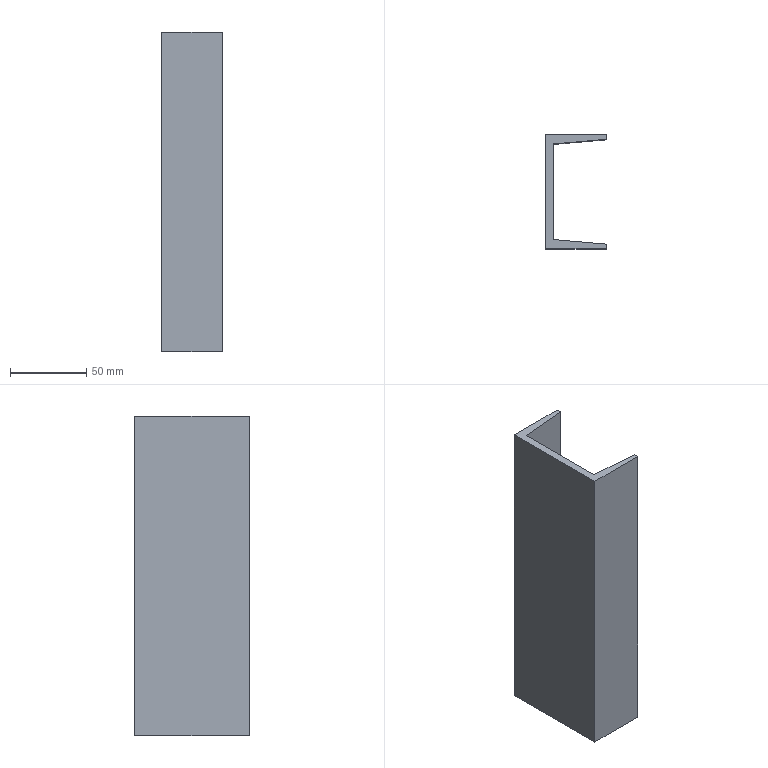Part | STEP file | BCC3 H13_7 | 1 solid | 12 faces | box 40 x 75 x 210 mm | volume 144819 mm3 | plane 10 | cylinder 2 | commonest cylinder face diameters 12 x2
STEP:
#1=CARTESIAN_POINT('',(0.,0.,0.));
#2=DIRECTION('',(0.,0.,1.));
#3=DIRECTION('',(1.,0.,0.));
#4=AXIS2_PLACEMENT_3D('',#1,#2,#3);
#5=CARTESIAN_POINT('',(20.,32.75,6.));
#6=VERTEX_POINT('',#5);
#7=CARTESIAN_POINT('',(20.,37.5,6.));
#8=VERTEX_POINT('',#7);
#9=CARTESIAN_POINT('',(20.,27.5,6.));
#10=DIRECTION('',(0.,1.,0.));
#11=VECTOR('',#10,1.);
#12=LINE('',#9,#11);
#13=CARTESIAN_POINT('',(20.,27.5,0.));
#14=DIRECTION('',(0.,1.,0.));
#15=DIRECTION('',(0.,0.,1.));
#16=AXIS2_PLACEMENT_3D('',#13,#14,#15);
#17=CYLINDRICAL_SURFACE('',#16,6.);
#18=CARTESIAN_POINT('',(6.283,0.));
#19=DIRECTION('',(0.,1.));
#20=VECTOR('',#19,1.);
#21=LINE('',#18,#20);
#22=(GEOMETRIC_REPRESENTATION_CONTEXT(2)PARAMETRIC_REPRESENTATION_CONTEXT()REPRESENTATION_CONTEXT('',''));
#23=DEFINITIONAL_REPRESENTATION('',(#21),#22);
#24=PCURVE('',#17,#23);
#25=CARTESIAN_POINT('',(20.,27.5,0.));
#26=DIRECTION('',(0.,1.,0.));
#27=DIRECTION('',(0.,0.,1.));
#28=AXIS2_PLACEMENT_3D('',#25,#26,#27);
#29=CYLINDRICAL_SURFACE('',#28,6.);
#30=CARTESIAN_POINT('',(0.,0.));
#31=DIRECTION('',(0.,1.));
#32=VECTOR('',#31,1.);
#33=LINE('',#30,#32);
#34=(GEOMETRIC_REPRESENTATION_CONTEXT(2)PARAMETRIC_REPRESENTATION_CONTEXT()REPRESENTATION_CONTEXT('',''));
#35=DEFINITIONAL_REPRESENTATION('',(#33),#34);
#36=PCURVE('',#29,#35);
#37=SURFACE_CURVE('',#12,(#24,#36),.PCURVE_S1.);
#38=EDGE_CURVE('',#6,#8,#37,.T.);
#39=ORIENTED_EDGE('',*,*,#38,.T.);
#40=CARTESIAN_POINT('',(20.,37.5,-6.));
#41=VERTEX_POINT('',#40);
#42=CARTESIAN_POINT('',(20.,37.5,0.));
#43=DIRECTION('',(0.,-1.,0.));
#44=DIRECTION('',(0.,0.,-1.));
#45=AXIS2_PLACEMENT_3D('',#42,#43,#44);
#46=CIRCLE('',#45,6.);
#47=CARTESIAN_POINT('',(9.425,10.));
#48=DIRECTION('',(-1.,0.));
#49=VECTOR('',#48,1.);
#50=LINE('',#47,#49);
#51=(GEOMETRIC_REPRESENTATION_CONTEXT(2)PARAMETRIC_REPRESENTATION_CONTEXT()REPRESENTATION_CONTEXT('',''));
#52=DEFINITIONAL_REPRESENTATION('',(#50),#51);
#53=PCURVE('',#17,#52);
#54=CARTESIAN_POINT('',(40.,37.5,105.));
#55=DIRECTION('',(0.,-1.,0.));
#56=DIRECTION('',(0.,0.,-1.));
#57=AXIS2_PLACEMENT_3D('',#54,#55,#56);
#58=PLANE('',#57);
#59=CARTESIAN_POINT('',(105.,-20.));
#60=DIRECTION('',(1.,0.));
#61=AXIS2_PLACEMENT_2D('',#59,#60);
#62=CIRCLE('',#61,6.);
#63=(GEOMETRIC_REPRESENTATION_CONTEXT(2)PARAMETRIC_REPRESENTATION_CONTEXT()REPRESENTATION_CONTEXT('',''));
#64=DEFINITIONAL_REPRESENTATION('',(#62),#63);
#65=PCURVE('',#58,#64);
#66=SURFACE_CURVE('',#46,(#53,#65),.PCURVE_S1.);
#67=EDGE_CURVE('',#8,#41,#66,.T.);
#68=ORIENTED_EDGE('',*,*,#67,.T.);
#69=CARTESIAN_POINT('',(20.,32.75,-6.));
#70=VERTEX_POINT('',#69);
#71=CARTESIAN_POINT('',(20.,27.5,-6.));
#72=DIRECTION('',(0.,1.,0.));
#73=VECTOR('',#72,1.);
#74=LINE('',#71,#73);
#75=CARTESIAN_POINT('',(3.142,0.));
#76=DIRECTION('',(0.,1.));
#77=VECTOR('',#76,1.);
#78=LINE('',#75,#77);
#79=(GEOMETRIC_REPRESENTATION_CONTEXT(2)PARAMETRIC_REPRESENTATION_CONTEXT()REPRESENTATION_CONTEXT('',''));
#80=DEFINITIONAL_REPRESENTATION('',(#78),#79);
#81=PCURVE('',#17,#80);
#82=CARTESIAN_POINT('',(3.142,0.));
#83=DIRECTION('',(0.,1.));
#84=VECTOR('',#83,1.);
#85=LINE('',#82,#84);
#86=(GEOMETRIC_REPRESENTATION_CONTEXT(2)PARAMETRIC_REPRESENTATION_CONTEXT()REPRESENTATION_CONTEXT('',''));
#87=DEFINITIONAL_REPRESENTATION('',(#85),#86);
#88=PCURVE('',#29,#87);
#89=SURFACE_CURVE('',#74,(#81,#88),.PCURVE_S1.);
#90=EDGE_CURVE('',#70,#41,#89,.T.);
#91=ORIENTED_EDGE('',*,*,#90,.F.);
#92=CARTESIAN_POINT('',(20.,32.75,6.));
#93=CARTESIAN_POINT('',(8.,31.7,6.));
#94=CARTESIAN_POINT('',(8.,31.7,-6.));
#95=CARTESIAN_POINT('',(20.,32.75,-6.));
#96=(BOUNDED_CURVE()B_SPLINE_CURVE(3,(#92,#93,#94,#95),.UNSPECIFIED.,.F.,.F.)B_SPLINE_CURVE_WITH_KNOTS((4,4),(1.571,4.712),.PIECEWISE_BEZIER_KNOTS.)CURVE()GEOMETRIC_REPRESENTATION_ITEM()RATIONAL_B_SPLINE_CURVE((1.,0.3333,0.3333,1.))REPRESENTATION_ITEM(''));
#97=CARTESIAN_POINT('',(6.283,5.25));
#98=CARTESIAN_POINT('',(6.253,5.234));
#99=CARTESIAN_POINT('',(6.19,5.201));
#100=CARTESIAN_POINT('',(6.085,5.147));
#101=CARTESIAN_POINT('',(5.972,5.089));
#102=CARTESIAN_POINT('',(5.848,5.028));
#103=CARTESIAN_POINT('',(5.713,4.966));
#104=CARTESIAN_POINT('',(5.567,4.904));
#105=CARTESIAN_POINT('',(5.412,4.847));
#106=CARTESIAN_POINT('',(5.246,4.796));
#107=CARTESIAN_POINT('',(5.073,4.757));
#108=CARTESIAN_POINT('',(4.894,4.731));
#109=CARTESIAN_POINT('',(4.712,4.722));
#110=CARTESIAN_POINT('',(4.531,4.731));
#111=CARTESIAN_POINT('',(4.352,4.757));
#112=CARTESIAN_POINT('',(4.179,4.796));
#113=CARTESIAN_POINT('',(4.013,4.847));
#114=CARTESIAN_POINT('',(3.857,4.904));
#115=CARTESIAN_POINT('',(3.712,4.966));
#116=CARTESIAN_POINT('',(3.577,5.028));
#117=CARTESIAN_POINT('',(3.453,5.089));
#118=CARTESIAN_POINT('',(3.339,5.147));
#119=CARTESIAN_POINT('',(3.235,5.201));
#120=CARTESIAN_POINT('',(3.172,5.234));
#121=CARTESIAN_POINT('',(3.142,5.25));
#122=B_SPLINE_CURVE_WITH_KNOTS('',3,(#97,#98,#99,#100,#101,#102,#103,#104,#105,#106,#107,#108,#109,#110,#111,#112,#113,#114,#115,#116,#117,#118,#119,#120,#121),.UNSPECIFIED.,.F.,.F.,(4,1,1,1,1,1,1,1,1,1,1,1,1,1,1,1,1,1,1,1,1,1,4),(1.571,1.714,1.856,1.999,2.142,2.285,2.428,2.57,2.713,2.856,2.999,3.142,3.284,3.427,3.57,3.713,3.856,3.998,4.141,4.284,4.427,4.57,4.712),.QUASI_UNIFORM_KNOTS.);
#123=(GEOMETRIC_REPRESENTATION_CONTEXT(2)PARAMETRIC_REPRESENTATION_CONTEXT()REPRESENTATION_CONTEXT('',''));
#124=DEFINITIONAL_REPRESENTATION('',(#122),#123);
#125=PCURVE('',#17,#124);
#126=CARTESIAN_POINT('',(5.,31.438,105.));
#127=DIRECTION('',(-0.08716,0.9962,0.));
#128=DIRECTION('',(-0.9962,-0.08716,0.));
#129=AXIS2_PLACEMENT_3D('',#126,#127,#128);
#130=PLANE('',#129);
#131=CARTESIAN_POINT('',(-15.057,-99.));
#132=CARTESIAN_POINT('',(-3.011,-99.));
#133=CARTESIAN_POINT('',(-3.011,-111.));
#134=CARTESIAN_POINT('',(-15.057,-111.));
#135=(BOUNDED_CURVE()B_SPLINE_CURVE(3,(#131,#132,#133,#134),.UNSPECIFIED.,.F.,.F.)B_SPLINE_CURVE_WITH_KNOTS((4,4),(1.571,4.712),.PIECEWISE_BEZIER_KNOTS.)CURVE()GEOMETRIC_REPRESENTATION_ITEM()RATIONAL_B_SPLINE_CURVE((1.,0.3333,0.3333,1.))REPRESENTATION_ITEM(''));
#136=(GEOMETRIC_REPRESENTATION_CONTEXT(2)PARAMETRIC_REPRESENTATION_CONTEXT()REPRESENTATION_CONTEXT('',''));
#137=DEFINITIONAL_REPRESENTATION('',(#135),#136);
#138=PCURVE('',#130,#137);
#139=SURFACE_CURVE('',#96,(#125,#138),.PCURVE_S1.);
#140=EDGE_CURVE('',#6,#70,#139,.T.);
#141=ORIENTED_EDGE('',*,*,#140,.F.);
#142=EDGE_LOOP('',(#39,#68,#91,#141));
#143=FACE_BOUND('',#142,.F.);
#144=ADVANCED_FACE('',(#143),#17,.F.);
#145=CARTESIAN_POINT('',(40.,37.5,-105.));
#146=VERTEX_POINT('',#145);
#147=CARTESIAN_POINT('',(0.,37.5,-105.));
#148=VERTEX_POINT('',#147);
#149=CARTESIAN_POINT('',(40.,37.5,-105.));
#150=DIRECTION('',(-1.,0.,0.));
#151=VECTOR('',#150,1.);
#152=LINE('',#149,#151);
#153=CARTESIAN_POINT('',(210.,0.));
#154=DIRECTION('',(0.,-1.));
#155=VECTOR('',#154,1.);
#156=LINE('',#153,#155);
#157=(GEOMETRIC_REPRESENTATION_CONTEXT(2)PARAMETRIC_REPRESENTATION_CONTEXT()REPRESENTATION_CONTEXT('',''));
#158=DEFINITIONAL_REPRESENTATION('',(#156),#157);
#159=PCURVE('',#58,#158);
#160=CARTESIAN_POINT('',(0.,0.,-105.));
#161=DIRECTION('',(0.,0.,1.));
#162=DIRECTION('',(1.,0.,0.));
#163=AXIS2_PLACEMENT_3D('',#160,#161,#162);
#164=PLANE('',#163);
#165=CARTESIAN_POINT('',(40.,37.5));
#166=DIRECTION('',(-1.,0.));
#167=VECTOR('',#166,1.);
#168=LINE('',#165,#167);
#169=(GEOMETRIC_REPRESENTATION_CONTEXT(2)PARAMETRIC_REPRESENTATION_CONTEXT()REPRESENTATION_CONTEXT('',''));
#170=DEFINITIONAL_REPRESENTATION('',(#168),#169);
#171=PCURVE('',#164,#170);
#172=SURFACE_CURVE('',#152,(#159,#171),.PCURVE_S1.);
#173=EDGE_CURVE('',#146,#148,#172,.T.);
#174=ORIENTED_EDGE('',*,*,#173,.T.);
#175=CARTESIAN_POINT('',(0.,37.5,105.));
#176=VERTEX_POINT('',#175);
#177=CARTESIAN_POINT('',(0.,37.5,105.));
#178=DIRECTION('',(0.,0.,-1.));
#179=VECTOR('',#178,1.);
#180=LINE('',#177,#179);
#181=CARTESIAN_POINT('',(0.,-40.));
#182=DIRECTION('',(1.,0.));
#183=VECTOR('',#182,1.);
#184=LINE('',#181,#183);
#185=(GEOMETRIC_REPRESENTATION_CONTEXT(2)PARAMETRIC_REPRESENTATION_CONTEXT()REPRESENTATION_CONTEXT('',''));
#186=DEFINITIONAL_REPRESENTATION('',(#184),#185);
#187=PCURVE('',#58,#186);
#188=CARTESIAN_POINT('',(0.,37.5,105.));
#189=DIRECTION('',(1.,0.,0.));
#190=DIRECTION('',(0.,0.,-1.));
#191=AXIS2_PLACEMENT_3D('',#188,#189,#190);
#192=PLANE('',#191);
#193=CARTESIAN_POINT('',(0.,0.));
#194=DIRECTION('',(1.,0.));
#195=VECTOR('',#194,1.);
#196=LINE('',#193,#195);
#197=(GEOMETRIC_REPRESENTATION_CONTEXT(2)PARAMETRIC_REPRESENTATION_CONTEXT()REPRESENTATION_CONTEXT('',''));
#198=DEFINITIONAL_REPRESENTATION('',(#196),#197);
#199=PCURVE('',#192,#198);
#200=SURFACE_CURVE('',#180,(#187,#199),.PCURVE_S1.);
#201=EDGE_CURVE('',#176,#148,#200,.T.);
#202=ORIENTED_EDGE('',*,*,#201,.F.);
#203=CARTESIAN_POINT('',(40.,37.5,105.));
#204=VERTEX_POINT('',#203);
#205=CARTESIAN_POINT('',(40.,37.5,105.));
#206=DIRECTION('',(-1.,0.,0.));
#207=VECTOR('',#206,1.);
#208=LINE('',#205,#207);
#209=CARTESIAN_POINT('',(0.,0.));
#210=DIRECTION('',(0.,-1.));
#211=VECTOR('',#210,1.);
#212=LINE('',#209,#211);
#213=(GEOMETRIC_REPRESENTATION_CONTEXT(2)PARAMETRIC_REPRESENTATION_CONTEXT()REPRESENTATION_CONTEXT('',''));
#214=DEFINITIONAL_REPRESENTATION('',(#212),#213);
#215=PCURVE('',#58,#214);
#216=CARTESIAN_POINT('',(0.,0.,105.));
#217=DIRECTION('',(0.,0.,1.));
#218=DIRECTION('',(1.,0.,0.));
#219=AXIS2_PLACEMENT_3D('',#216,#217,#218);
#220=PLANE('',#219);
#221=CARTESIAN_POINT('',(40.,37.5));
#222=DIRECTION('',(-1.,0.));
#223=VECTOR('',#222,1.);
#224=LINE('',#221,#223);
#225=(GEOMETRIC_REPRESENTATION_CONTEXT(2)PARAMETRIC_REPRESENTATION_CONTEXT()REPRESENTATION_CONTEXT('',''));
#226=DEFINITIONAL_REPRESENTATION('',(#224),#225);
#227=PCURVE('',#220,#226);
#228=SURFACE_CURVE('',#208,(#215,#227),.PCURVE_S1.);
#229=EDGE_CURVE('',#204,#176,#228,.T.);
#230=ORIENTED_EDGE('',*,*,#229,.F.);
#231=CARTESIAN_POINT('',(40.,37.5,105.));
#232=DIRECTION('',(0.,0.,-1.));
#233=VECTOR('',#232,1.);
#234=LINE('',#231,#233);
#235=CARTESIAN_POINT('',(0.,0.));
#236=DIRECTION('',(1.,0.));
#237=VECTOR('',#236,1.);
#238=LINE('',#235,#237);
#239=(GEOMETRIC_REPRESENTATION_CONTEXT(2)PARAMETRIC_REPRESENTATION_CONTEXT()REPRESENTATION_CONTEXT('',''));
#240=DEFINITIONAL_REPRESENTATION('',(#238),#239);
#241=PCURVE('',#58,#240);
#242=CARTESIAN_POINT('',(40.,34.5,105.));
#243=DIRECTION('',(-1.,0.,0.));
#244=DIRECTION('',(0.,0.,1.));
#245=AXIS2_PLACEMENT_3D('',#242,#243,#244);
#246=PLANE('',#245);
#247=CARTESIAN_POINT('',(0.,3.));
#248=DIRECTION('',(-1.,0.));
#249=VECTOR('',#248,1.);
#250=LINE('',#247,#249);
#251=(GEOMETRIC_REPRESENTATION_CONTEXT(2)PARAMETRIC_REPRESENTATION_CONTEXT()REPRESENTATION_CONTEXT('',''));
#252=DEFINITIONAL_REPRESENTATION('',(#250),#251);
#253=PCURVE('',#246,#252);
#254=SURFACE_CURVE('',#234,(#241,#253),.PCURVE_S1.);
#255=EDGE_CURVE('',#204,#146,#254,.T.);
#256=ORIENTED_EDGE('',*,*,#255,.T.);
#257=EDGE_LOOP('',(#174,#202,#230,#256));
#258=FACE_BOUND('',#257,.T.);
#259=ORIENTED_EDGE('',*,*,#67,.T.);
#260=CARTESIAN_POINT('',(20.,37.5,0.));
#261=DIRECTION('',(0.,-1.,0.));
#262=DIRECTION('',(0.,0.,-1.));
#263=AXIS2_PLACEMENT_3D('',#260,#261,#262);
#264=CIRCLE('',#263,6.);
#265=CARTESIAN_POINT('',(105.,-20.));
#266=DIRECTION('',(1.,0.));
#267=AXIS2_PLACEMENT_2D('',#265,#266);
#268=CIRCLE('',#267,6.);
#269=(GEOMETRIC_REPRESENTATION_CONTEXT(2)PARAMETRIC_REPRESENTATION_CONTEXT()REPRESENTATION_CONTEXT('',''));
#270=DEFINITIONAL_REPRESENTATION('',(#268),#269);
#271=PCURVE('',#58,#270);
#272=CARTESIAN_POINT('',(3.142,10.));
#273=DIRECTION('',(-1.,0.));
#274=VECTOR('',#273,1.);
#275=LINE('',#272,#274);
#276=(GEOMETRIC_REPRESENTATION_CONTEXT(2)PARAMETRIC_REPRESENTATION_CONTEXT()REPRESENTATION_CONTEXT('',''));
#277=DEFINITIONAL_REPRESENTATION('',(#275),#276);
#278=PCURVE('',#29,#277);
#279=SURFACE_CURVE('',#264,(#271,#278),.PCURVE_S1.);
#280=EDGE_CURVE('',#41,#8,#279,.T.);
#281=ORIENTED_EDGE('',*,*,#280,.T.);
#282=EDGE_LOOP('',(#259,#281));
#283=FACE_BOUND('',#282,.T.);
#284=ADVANCED_FACE('',(#258,#283),#58,.F.);
#285=CARTESIAN_POINT('',(5.,31.438,-105.));
#286=VERTEX_POINT('',#285);
#287=CARTESIAN_POINT('',(40.,34.5,-105.));
#288=VERTEX_POINT('',#287);
#289=CARTESIAN_POINT('',(5.,31.438,-105.));
#290=DIRECTION('',(0.9962,0.08716,0.));
#291=VECTOR('',#290,1.);
#292=LINE('',#289,#291);
#293=CARTESIAN_POINT('',(0.,-210.));
#294=DIRECTION('',(-1.,0.));
#295=VECTOR('',#294,1.);
#296=LINE('',#293,#295);
#297=(GEOMETRIC_REPRESENTATION_CONTEXT(2)PARAMETRIC_REPRESENTATION_CONTEXT()REPRESENTATION_CONTEXT('',''));
#298=DEFINITIONAL_REPRESENTATION('',(#296),#297);
#299=PCURVE('',#130,#298);
#300=CARTESIAN_POINT('',(5.,31.438));
#301=DIRECTION('',(0.9962,0.08716));
#302=VECTOR('',#301,1.);
#303=LINE('',#300,#302);
#304=(GEOMETRIC_REPRESENTATION_CONTEXT(2)PARAMETRIC_REPRESENTATION_CONTEXT()REPRESENTATION_CONTEXT('',''));
#305=DEFINITIONAL_REPRESENTATION('',(#303),#304);
#306=PCURVE('',#164,#305);
#307=SURFACE_CURVE('',#292,(#299,#306),.PCURVE_S1.);
#308=EDGE_CURVE('',#286,#288,#307,.T.);
#309=ORIENTED_EDGE('',*,*,#308,.T.);
#310=CARTESIAN_POINT('',(40.,34.5,105.));
#311=VERTEX_POINT('',#310);
#312=CARTESIAN_POINT('',(40.,34.5,105.));
#313=DIRECTION('',(0.,0.,-1.));
#314=VECTOR('',#313,1.);
#315=LINE('',#312,#314);
#316=CARTESIAN_POINT('',(-35.134,0.));
#317=DIRECTION('',(0.,-1.));
#318=VECTOR('',#317,1.);
#319=LINE('',#316,#318);
#320=(GEOMETRIC_REPRESENTATION_CONTEXT(2)PARAMETRIC_REPRESENTATION_CONTEXT()REPRESENTATION_CONTEXT('',''));
#321=DEFINITIONAL_REPRESENTATION('',(#319),#320);
#322=PCURVE('',#130,#321);
#323=CARTESIAN_POINT('',(0.,0.));
#324=DIRECTION('',(-1.,0.));
#325=VECTOR('',#324,1.);
#326=LINE('',#323,#325);
#327=(GEOMETRIC_REPRESENTATION_CONTEXT(2)PARAMETRIC_REPRESENTATION_CONTEXT()REPRESENTATION_CONTEXT('',''));
#328=DEFINITIONAL_REPRESENTATION('',(#326),#327);
#329=PCURVE('',#246,#328);
#330=SURFACE_CURVE('',#315,(#322,#329),.PCURVE_S1.);
#331=EDGE_CURVE('',#311,#288,#330,.T.);
#332=ORIENTED_EDGE('',*,*,#331,.F.);
#333=CARTESIAN_POINT('',(5.,31.438,105.));
#334=VERTEX_POINT('',#333);
#335=CARTESIAN_POINT('',(5.,31.438,105.));
#336=DIRECTION('',(0.9962,0.08716,0.));
#337=VECTOR('',#336,1.);
#338=LINE('',#335,#337);
#339=CARTESIAN_POINT('',(0.,0.));
#340=DIRECTION('',(-1.,0.));
#341=VECTOR('',#340,1.);
#342=LINE('',#339,#341);
#343=(GEOMETRIC_REPRESENTATION_CONTEXT(2)PARAMETRIC_REPRESENTATION_CONTEXT()REPRESENTATION_CONTEXT('',''));
#344=DEFINITIONAL_REPRESENTATION('',(#342),#343);
#345=PCURVE('',#130,#344);
#346=CARTESIAN_POINT('',(5.,31.438));
#347=DIRECTION('',(0.9962,0.08716));
#348=VECTOR('',#347,1.);
#349=LINE('',#346,#348);
#350=(GEOMETRIC_REPRESENTATION_CONTEXT(2)PARAMETRIC_REPRESENTATION_CONTEXT()REPRESENTATION_CONTEXT('',''));
#351=DEFINITIONAL_REPRESENTATION('',(#349),#350);
#352=PCURVE('',#220,#351);
#353=SURFACE_CURVE('',#338,(#345,#352),.PCURVE_S1.);
#354=EDGE_CURVE('',#334,#311,#353,.T.);
#355=ORIENTED_EDGE('',*,*,#354,.F.);
#356=CARTESIAN_POINT('',(5.,31.438,105.));
#357=DIRECTION('',(0.,0.,-1.));
#358=VECTOR('',#357,1.);
#359=LINE('',#356,#358);
#360=CARTESIAN_POINT('',(0.,0.));
#361=DIRECTION('',(0.,-1.));
#362=VECTOR('',#361,1.);
#363=LINE('',#360,#362);
#364=(GEOMETRIC_REPRESENTATION_CONTEXT(2)PARAMETRIC_REPRESENTATION_CONTEXT()REPRESENTATION_CONTEXT('',''));
#365=DEFINITIONAL_REPRESENTATION('',(#363),#364);
#366=PCURVE('',#130,#365);
#367=CARTESIAN_POINT('',(5.,-31.438,105.));
#368=DIRECTION('',(-1.,0.,0.));
#369=DIRECTION('',(0.,0.,1.));
#370=AXIS2_PLACEMENT_3D('',#367,#368,#369);
#371=PLANE('',#370);
#372=CARTESIAN_POINT('',(0.,62.876));
#373=DIRECTION('',(-1.,0.));
#374=VECTOR('',#373,1.);
#375=LINE('',#372,#374);
#376=(GEOMETRIC_REPRESENTATION_CONTEXT(2)PARAMETRIC_REPRESENTATION_CONTEXT()REPRESENTATION_CONTEXT('',''));
#377=DEFINITIONAL_REPRESENTATION('',(#375),#376);
#378=PCURVE('',#371,#377);
#379=SURFACE_CURVE('',#359,(#366,#378),.PCURVE_S1.);
#380=EDGE_CURVE('',#334,#286,#379,.T.);
#381=ORIENTED_EDGE('',*,*,#380,.T.);
#382=EDGE_LOOP('',(#309,#332,#355,#381));
#383=FACE_BOUND('',#382,.T.);
#384=ORIENTED_EDGE('',*,*,#140,.F.);
#385=CARTESIAN_POINT('',(20.,32.75,-6.));
#386=CARTESIAN_POINT('',(32.,33.8,-6.));
#387=CARTESIAN_POINT('',(32.,33.8,6.));
#388=CARTESIAN_POINT('',(20.,32.75,6.));
#389=(BOUNDED_CURVE()B_SPLINE_CURVE(3,(#385,#386,#387,#388),.UNSPECIFIED.,.F.,.F.)B_SPLINE_CURVE_WITH_KNOTS((4,4),(4.712,7.854),.PIECEWISE_BEZIER_KNOTS.)CURVE()GEOMETRIC_REPRESENTATION_ITEM()RATIONAL_B_SPLINE_CURVE((1.,0.3333,0.3333,1.))REPRESENTATION_ITEM(''));
#390=CARTESIAN_POINT('',(-15.057,-111.));
#391=CARTESIAN_POINT('',(-27.103,-111.));
#392=CARTESIAN_POINT('',(-27.103,-99.));
#393=CARTESIAN_POINT('',(-15.057,-99.));
#394=(BOUNDED_CURVE()B_SPLINE_CURVE(3,(#390,#391,#392,#393),.UNSPECIFIED.,.F.,.F.)B_SPLINE_CURVE_WITH_KNOTS((4,4),(4.712,7.854),.PIECEWISE_BEZIER_KNOTS.)CURVE()GEOMETRIC_REPRESENTATION_ITEM()RATIONAL_B_SPLINE_CURVE((1.,0.3333,0.3333,1.))REPRESENTATION_ITEM(''));
#395=(GEOMETRIC_REPRESENTATION_CONTEXT(2)PARAMETRIC_REPRESENTATION_CONTEXT()REPRESENTATION_CONTEXT('',''));
#396=DEFINITIONAL_REPRESENTATION('',(#394),#395);
#397=PCURVE('',#130,#396);
#398=CARTESIAN_POINT('',(3.142,5.25));
#399=CARTESIAN_POINT('',(3.111,5.266));
#400=CARTESIAN_POINT('',(3.048,5.299));
#401=CARTESIAN_POINT('',(2.944,5.354));
#402=CARTESIAN_POINT('',(2.83,5.411));
#403=CARTESIAN_POINT('',(2.706,5.472));
#404=CARTESIAN_POINT('',(2.571,5.535));
#405=CARTESIAN_POINT('',(2.426,5.596));
#406=CARTESIAN_POINT('',(2.27,5.654));
#407=CARTESIAN_POINT('',(2.105,5.704));
#408=CARTESIAN_POINT('',(1.931,5.744));
#409=CARTESIAN_POINT('',(1.753,5.769));
#410=CARTESIAN_POINT('',(1.571,5.778));
#411=CARTESIAN_POINT('',(1.389,5.769));
#412=CARTESIAN_POINT('',(1.21,5.744));
#413=CARTESIAN_POINT('',(1.037,5.704));
#414=CARTESIAN_POINT('',(0.8717,5.654));
#415=CARTESIAN_POINT('',(0.7158,5.596));
#416=CARTESIAN_POINT('',(0.5703,5.535));
#417=CARTESIAN_POINT('',(0.4356,5.472));
#418=CARTESIAN_POINT('',(0.3115,5.411));
#419=CARTESIAN_POINT('',(0.1977,5.354));
#420=CARTESIAN_POINT('',(0.09367,5.299));
#421=CARTESIAN_POINT('',(0.0303,5.266));
#422=CARTESIAN_POINT('',(0.,5.25));
#423=B_SPLINE_CURVE_WITH_KNOTS('',3,(#398,#399,#400,#401,#402,#403,#404,#405,#406,#407,#408,#409,#410,#411,#412,#413,#414,#415,#416,#417,#418,#419,#420,#421,#422),.UNSPECIFIED.,.F.,.F.,(4,1,1,1,1,1,1,1,1,1,1,1,1,1,1,1,1,1,1,1,1,1,4),(4.712,4.855,4.998,5.141,5.284,5.426,5.569,5.712,5.855,5.998,6.14,6.283,6.426,6.569,6.712,6.854,6.997,7.14,7.283,7.426,7.568,7.711,7.854),.QUASI_UNIFORM_KNOTS.);
#424=(GEOMETRIC_REPRESENTATION_CONTEXT(2)PARAMETRIC_REPRESENTATION_CONTEXT()REPRESENTATION_CONTEXT('',''));
#425=DEFINITIONAL_REPRESENTATION('',(#423),#424);
#426=PCURVE('',#29,#425);
#427=SURFACE_CURVE('',#389,(#397,#426),.PCURVE_S1.);
#428=EDGE_CURVE('',#70,#6,#427,.T.);
#429=ORIENTED_EDGE('',*,*,#428,.F.);
#430=EDGE_LOOP('',(#384,#429));
#431=FACE_BOUND('',#430,.T.);
#432=ADVANCED_FACE('',(#383,#431),#130,.F.);
#433=CARTESIAN_POINT('',(0.,-37.5,-105.));
#434=VERTEX_POINT('',#433);
#435=CARTESIAN_POINT('',(0.,37.5,-105.));
#436=DIRECTION('',(0.,-1.,0.));
#437=VECTOR('',#436,1.);
#438=LINE('',#435,#437);
#439=CARTESIAN_POINT('',(210.,0.));
#440=DIRECTION('',(0.,-1.));
#441=VECTOR('',#440,1.);
#442=LINE('',#439,#441);
#443=(GEOMETRIC_REPRESENTATION_CONTEXT(2)PARAMETRIC_REPRESENTATION_CONTEXT()REPRESENTATION_CONTEXT('',''));
#444=DEFINITIONAL_REPRESENTATION('',(#442),#443);
#445=PCURVE('',#192,#444);
#446=CARTESIAN_POINT('',(0.,37.5));
#447=DIRECTION('',(0.,-1.));
#448=VECTOR('',#447,1.);
#449=LINE('',#446,#448);
#450=(GEOMETRIC_REPRESENTATION_CONTEXT(2)PARAMETRIC_REPRESENTATION_CONTEXT()REPRESENTATION_CONTEXT('',''));
#451=DEFINITIONAL_REPRESENTATION('',(#449),#450);
#452=PCURVE('',#164,#451);
#453=SURFACE_CURVE('',#438,(#445,#452),.PCURVE_S1.);
#454=EDGE_CURVE('',#148,#434,#453,.T.);
#455=ORIENTED_EDGE('',*,*,#454,.T.);
#456=CARTESIAN_POINT('',(0.,-37.5,105.));
#457=VERTEX_POINT('',#456);
#458=CARTESIAN_POINT('',(0.,-37.5,105.));
#459=DIRECTION('',(0.,0.,-1.));
#460=VECTOR('',#459,1.);
#461=LINE('',#458,#460);
#462=CARTESIAN_POINT('',(0.,-75.));
#463=DIRECTION('',(1.,0.));
#464=VECTOR('',#463,1.);
#465=LINE('',#462,#464);
#466=(GEOMETRIC_REPRESENTATION_CONTEXT(2)PARAMETRIC_REPRESENTATION_CONTEXT()REPRESENTATION_CONTEXT('',''));
#467=DEFINITIONAL_REPRESENTATION('',(#465),#466);
#468=PCURVE('',#192,#467);
#469=CARTESIAN_POINT('',(0.,-37.5,105.));
#470=DIRECTION('',(0.,1.,0.));
#471=DIRECTION('',(0.,0.,1.));
#472=AXIS2_PLACEMENT_3D('',#469,#470,#471);
#473=PLANE('',#472);
#474=CARTESIAN_POINT('',(0.,0.));
#475=DIRECTION('',(-1.,0.));
#476=VECTOR('',#475,1.);
#477=LINE('',#474,#476);
#478=(GEOMETRIC_REPRESENTATION_CONTEXT(2)PARAMETRIC_REPRESENTATION_CONTEXT()REPRESENTATION_CONTEXT('',''));
#479=DEFINITIONAL_REPRESENTATION('',(#477),#478);
#480=PCURVE('',#473,#479);
#481=SURFACE_CURVE('',#461,(#468,#480),.PCURVE_S1.);
#482=EDGE_CURVE('',#457,#434,#481,.T.);
#483=ORIENTED_EDGE('',*,*,#482,.F.);
#484=CARTESIAN_POINT('',(0.,37.5,105.));
#485=DIRECTION('',(0.,-1.,0.));
#486=VECTOR('',#485,1.);
#487=LINE('',#484,#486);
#488=CARTESIAN_POINT('',(0.,0.));
#489=DIRECTION('',(0.,-1.));
#490=VECTOR('',#489,1.);
#491=LINE('',#488,#490);
#492=(GEOMETRIC_REPRESENTATION_CONTEXT(2)PARAMETRIC_REPRESENTATION_CONTEXT()REPRESENTATION_CONTEXT('',''));
#493=DEFINITIONAL_REPRESENTATION('',(#491),#492);
#494=PCURVE('',#192,#493);
#495=CARTESIAN_POINT('',(0.,37.5));
#496=DIRECTION('',(0.,-1.));
#497=VECTOR('',#496,1.);
#498=LINE('',#495,#497);
#499=(GEOMETRIC_REPRESENTATION_CONTEXT(2)PARAMETRIC_REPRESENTATION_CONTEXT()REPRESENTATION_CONTEXT('',''));
#500=DEFINITIONAL_REPRESENTATION('',(#498),#499);
#501=PCURVE('',#220,#500);
#502=SURFACE_CURVE('',#487,(#494,#501),.PCURVE_S1.);
#503=EDGE_CURVE('',#176,#457,#502,.T.);
#504=ORIENTED_EDGE('',*,*,#503,.F.);
#505=ORIENTED_EDGE('',*,*,#201,.T.);
#506=EDGE_LOOP('',(#455,#483,#504,#505));
#507=FACE_BOUND('',#506,.T.);
#508=ADVANCED_FACE('',(#507),#192,.F.);
#509=CARTESIAN_POINT('',(40.,-37.5,-105.));
#510=VERTEX_POINT('',#509);
#511=CARTESIAN_POINT('',(0.,-37.5,-105.));
#512=DIRECTION('',(1.,0.,0.));
#513=VECTOR('',#512,1.);
#514=LINE('',#511,#513);
#515=CARTESIAN_POINT('',(-210.,0.));
#516=DIRECTION('',(0.,1.));
#517=VECTOR('',#516,1.);
#518=LINE('',#515,#517);
#519=(GEOMETRIC_REPRESENTATION_CONTEXT(2)PARAMETRIC_REPRESENTATION_CONTEXT()REPRESENTATION_CONTEXT('',''));
#520=DEFINITIONAL_REPRESENTATION('',(#518),#519);
#521=PCURVE('',#473,#520);
#522=CARTESIAN_POINT('',(0.,-37.5));
#523=DIRECTION('',(1.,0.));
#524=VECTOR('',#523,1.);
#525=LINE('',#522,#524);
#526=(GEOMETRIC_REPRESENTATION_CONTEXT(2)PARAMETRIC_REPRESENTATION_CONTEXT()REPRESENTATION_CONTEXT('',''));
#527=DEFINITIONAL_REPRESENTATION('',(#525),#526);
#528=PCURVE('',#164,#527);
#529=SURFACE_CURVE('',#514,(#521,#528),.PCURVE_S1.);
#530=EDGE_CURVE('',#434,#510,#529,.T.);
#531=ORIENTED_EDGE('',*,*,#530,.T.);
#532=CARTESIAN_POINT('',(40.,-37.5,105.));
#533=VERTEX_POINT('',#532);
#534=CARTESIAN_POINT('',(40.,-37.5,105.));
#535=DIRECTION('',(0.,0.,-1.));
#536=VECTOR('',#535,1.);
#537=LINE('',#534,#536);
#538=CARTESIAN_POINT('',(0.,40.));
#539=DIRECTION('',(-1.,0.));
#540=VECTOR('',#539,1.);
#541=LINE('',#538,#540);
#542=(GEOMETRIC_REPRESENTATION_CONTEXT(2)PARAMETRIC_REPRESENTATION_CONTEXT()REPRESENTATION_CONTEXT('',''));
#543=DEFINITIONAL_REPRESENTATION('',(#541),#542);
#544=PCURVE('',#473,#543);
#545=CARTESIAN_POINT('',(40.,-37.5,105.));
#546=DIRECTION('',(-1.,0.,0.));
#547=DIRECTION('',(0.,0.,1.));
#548=AXIS2_PLACEMENT_3D('',#545,#546,#547);
#549=PLANE('',#548);
#550=CARTESIAN_POINT('',(0.,0.));
#551=DIRECTION('',(-1.,0.));
#552=VECTOR('',#551,1.);
#553=LINE('',#550,#552);
#554=(GEOMETRIC_REPRESENTATION_CONTEXT(2)PARAMETRIC_REPRESENTATION_CONTEXT()REPRESENTATION_CONTEXT('',''));
#555=DEFINITIONAL_REPRESENTATION('',(#553),#554);
#556=PCURVE('',#549,#555);
#557=SURFACE_CURVE('',#537,(#544,#556),.PCURVE_S1.);
#558=EDGE_CURVE('',#533,#510,#557,.T.);
#559=ORIENTED_EDGE('',*,*,#558,.F.);
#560=CARTESIAN_POINT('',(0.,-37.5,105.));
#561=DIRECTION('',(1.,0.,0.));
#562=VECTOR('',#561,1.);
#563=LINE('',#560,#562);
#564=CARTESIAN_POINT('',(0.,0.));
#565=DIRECTION('',(0.,1.));
#566=VECTOR('',#565,1.);
#567=LINE('',#564,#566);
#568=(GEOMETRIC_REPRESENTATION_CONTEXT(2)PARAMETRIC_REPRESENTATION_CONTEXT()REPRESENTATION_CONTEXT('',''));
#569=DEFINITIONAL_REPRESENTATION('',(#567),#568);
#570=PCURVE('',#473,#569);
#571=CARTESIAN_POINT('',(0.,-37.5));
#572=DIRECTION('',(1.,0.));
#573=VECTOR('',#572,1.);
#574=LINE('',#571,#573);
#575=(GEOMETRIC_REPRESENTATION_CONTEXT(2)PARAMETRIC_REPRESENTATION_CONTEXT()REPRESENTATION_CONTEXT('',''));
#576=DEFINITIONAL_REPRESENTATION('',(#574),#575);
#577=PCURVE('',#220,#576);
#578=SURFACE_CURVE('',#563,(#570,#577),.PCURVE_S1.);
#579=EDGE_CURVE('',#457,#533,#578,.T.);
#580=ORIENTED_EDGE('',*,*,#579,.F.);
#581=ORIENTED_EDGE('',*,*,#482,.T.);
#582=EDGE_LOOP('',(#531,#559,#580,#581));
#583=FACE_BOUND('',#582,.T.);
#584=ADVANCED_FACE('',(#583),#473,.F.);
#585=CARTESIAN_POINT('',(40.,-34.5,-105.));
#586=VERTEX_POINT('',#585);
#587=CARTESIAN_POINT('',(40.,-37.5,-105.));
#588=DIRECTION('',(0.,1.,0.));
#589=VECTOR('',#588,1.);
#590=LINE('',#587,#589);
#591=CARTESIAN_POINT('',(-210.,0.));
#592=DIRECTION('',(0.,1.));
#593=VECTOR('',#592,1.);
#594=LINE('',#591,#593);
#595=(GEOMETRIC_REPRESENTATION_CONTEXT(2)PARAMETRIC_REPRESENTATION_CONTEXT()REPRESENTATION_CONTEXT('',''));
#596=DEFINITIONAL_REPRESENTATION('',(#594),#595);
#597=PCURVE('',#549,#596);
#598=CARTESIAN_POINT('',(40.,-37.5));
#599=DIRECTION('',(0.,1.));
#600=VECTOR('',#599,1.);
#601=LINE('',#598,#600);
#602=(GEOMETRIC_REPRESENTATION_CONTEXT(2)PARAMETRIC_REPRESENTATION_CONTEXT()REPRESENTATION_CONTEXT('',''));
#603=DEFINITIONAL_REPRESENTATION('',(#601),#602);
#604=PCURVE('',#164,#603);
#605=SURFACE_CURVE('',#590,(#597,#604),.PCURVE_S1.);
#606=EDGE_CURVE('',#510,#586,#605,.T.);
#607=ORIENTED_EDGE('',*,*,#606,.T.);
#608=CARTESIAN_POINT('',(40.,-34.5,105.));
#609=VERTEX_POINT('',#608);
#610=CARTESIAN_POINT('',(40.,-34.5,105.));
#611=DIRECTION('',(0.,0.,-1.));
#612=VECTOR('',#611,1.);
#613=LINE('',#610,#612);
#614=CARTESIAN_POINT('',(0.,3.));
#615=DIRECTION('',(-1.,0.));
#616=VECTOR('',#615,1.);
#617=LINE('',#614,#616);
#618=(GEOMETRIC_REPRESENTATION_CONTEXT(2)PARAMETRIC_REPRESENTATION_CONTEXT()REPRESENTATION_CONTEXT('',''));
#619=DEFINITIONAL_REPRESENTATION('',(#617),#618);
#620=PCURVE('',#549,#619);
#621=CARTESIAN_POINT('',(40.,-34.5,105.));
#622=DIRECTION('',(-0.08716,-0.9962,0.));
#623=DIRECTION('',(0.9962,-0.08716,0.));
#624=AXIS2_PLACEMENT_3D('',#621,#622,#623);
#625=PLANE('',#624);
#626=CARTESIAN_POINT('',(0.,0.));
#627=DIRECTION('',(0.,-1.));
#628=VECTOR('',#627,1.);
#629=LINE('',#626,#628);
#630=(GEOMETRIC_REPRESENTATION_CONTEXT(2)PARAMETRIC_REPRESENTATION_CONTEXT()REPRESENTATION_CONTEXT('',''));
#631=DEFINITIONAL_REPRESENTATION('',(#629),#630);
#632=PCURVE('',#625,#631);
#633=SURFACE_CURVE('',#613,(#620,#632),.PCURVE_S1.);
#634=EDGE_CURVE('',#609,#586,#633,.T.);
#635=ORIENTED_EDGE('',*,*,#634,.F.);
#636=CARTESIAN_POINT('',(40.,-37.5,105.));
#637=DIRECTION('',(0.,1.,0.));
#638=VECTOR('',#637,1.);
#639=LINE('',#636,#638);
#640=CARTESIAN_POINT('',(0.,0.));
#641=DIRECTION('',(0.,1.));
#642=VECTOR('',#641,1.);
#643=LINE('',#640,#642);
#644=(GEOMETRIC_REPRESENTATION_CONTEXT(2)PARAMETRIC_REPRESENTATION_CONTEXT()REPRESENTATION_CONTEXT('',''));
#645=DEFINITIONAL_REPRESENTATION('',(#643),#644);
#646=PCURVE('',#549,#645);
#647=CARTESIAN_POINT('',(40.,-37.5));
#648=DIRECTION('',(0.,1.));
#649=VECTOR('',#648,1.);
#650=LINE('',#647,#649);
#651=(GEOMETRIC_REPRESENTATION_CONTEXT(2)PARAMETRIC_REPRESENTATION_CONTEXT()REPRESENTATION_CONTEXT('',''));
#652=DEFINITIONAL_REPRESENTATION('',(#650),#651);
#653=PCURVE('',#220,#652);
#654=SURFACE_CURVE('',#639,(#646,#653),.PCURVE_S1.);
#655=EDGE_CURVE('',#533,#609,#654,.T.);
#656=ORIENTED_EDGE('',*,*,#655,.F.);
#657=ORIENTED_EDGE('',*,*,#558,.T.);
#658=EDGE_LOOP('',(#607,#635,#656,#657));
#659=FACE_BOUND('',#658,.T.);
#660=ADVANCED_FACE('',(#659),#549,.F.);
#661=CARTESIAN_POINT('',(5.,-31.438,-105.));
#662=VERTEX_POINT('',#661);
#663=CARTESIAN_POINT('',(40.,-34.5,-105.));
#664=DIRECTION('',(-0.9962,0.08716,0.));
#665=VECTOR('',#664,1.);
#666=LINE('',#663,#665);
#667=CARTESIAN_POINT('',(0.,-210.));
#668=DIRECTION('',(-1.,0.));
#669=VECTOR('',#668,1.);
#670=LINE('',#667,#669);
#671=(GEOMETRIC_REPRESENTATION_CONTEXT(2)PARAMETRIC_REPRESENTATION_CONTEXT()REPRESENTATION_CONTEXT('',''));
#672=DEFINITIONAL_REPRESENTATION('',(#670),#671);
#673=PCURVE('',#625,#672);
#674=CARTESIAN_POINT('',(40.,-34.5));
#675=DIRECTION('',(-0.9962,0.08716));
#676=VECTOR('',#675,1.);
#677=LINE('',#674,#676);
#678=(GEOMETRIC_REPRESENTATION_CONTEXT(2)PARAMETRIC_REPRESENTATION_CONTEXT()REPRESENTATION_CONTEXT('',''));
#679=DEFINITIONAL_REPRESENTATION('',(#677),#678);
#680=PCURVE('',#164,#679);
#681=SURFACE_CURVE('',#666,(#673,#680),.PCURVE_S1.);
#682=EDGE_CURVE('',#586,#662,#681,.T.);
#683=ORIENTED_EDGE('',*,*,#682,.T.);
#684=CARTESIAN_POINT('',(5.,-31.438,105.));
#685=VERTEX_POINT('',#684);
#686=CARTESIAN_POINT('',(5.,-31.438,105.));
#687=DIRECTION('',(0.,0.,-1.));
#688=VECTOR('',#687,1.);
#689=LINE('',#686,#688);
#690=CARTESIAN_POINT('',(-35.134,0.));
#691=DIRECTION('',(0.,-1.));
#692=VECTOR('',#691,1.);
#693=LINE('',#690,#692);
#694=(GEOMETRIC_REPRESENTATION_CONTEXT(2)PARAMETRIC_REPRESENTATION_CONTEXT()REPRESENTATION_CONTEXT('',''));
#695=DEFINITIONAL_REPRESENTATION('',(#693),#694);
#696=PCURVE('',#625,#695);
#697=CARTESIAN_POINT('',(0.,0.));
#698=DIRECTION('',(-1.,0.));
#699=VECTOR('',#698,1.);
#700=LINE('',#697,#699);
#701=(GEOMETRIC_REPRESENTATION_CONTEXT(2)PARAMETRIC_REPRESENTATION_CONTEXT()REPRESENTATION_CONTEXT('',''));
#702=DEFINITIONAL_REPRESENTATION('',(#700),#701);
#703=PCURVE('',#371,#702);
#704=SURFACE_CURVE('',#689,(#696,#703),.PCURVE_S1.);
#705=EDGE_CURVE('',#685,#662,#704,.T.);
#706=ORIENTED_EDGE('',*,*,#705,.F.);
#707=CARTESIAN_POINT('',(40.,-34.5,105.));
#708=DIRECTION('',(-0.9962,0.08716,0.));
#709=VECTOR('',#708,1.);
#710=LINE('',#707,#709);
#711=CARTESIAN_POINT('',(0.,0.));
#712=DIRECTION('',(-1.,0.));
#713=VECTOR('',#712,1.);
#714=LINE('',#711,#713);
#715=(GEOMETRIC_REPRESENTATION_CONTEXT(2)PARAMETRIC_REPRESENTATION_CONTEXT()REPRESENTATION_CONTEXT('',''));
#716=DEFINITIONAL_REPRESENTATION('',(#714),#715);
#717=PCURVE('',#625,#716);
#718=CARTESIAN_POINT('',(40.,-34.5));
#719=DIRECTION('',(-0.9962,0.08716));
#720=VECTOR('',#719,1.);
#721=LINE('',#718,#720);
#722=(GEOMETRIC_REPRESENTATION_CONTEXT(2)PARAMETRIC_REPRESENTATION_CONTEXT()REPRESENTATION_CONTEXT('',''));
#723=DEFINITIONAL_REPRESENTATION('',(#721),#722);
#724=PCURVE('',#220,#723);
#725=SURFACE_CURVE('',#710,(#717,#724),.PCURVE_S1.);
#726=EDGE_CURVE('',#609,#685,#725,.T.);
#727=ORIENTED_EDGE('',*,*,#726,.F.);
#728=ORIENTED_EDGE('',*,*,#634,.T.);
#729=EDGE_LOOP('',(#683,#706,#727,#728));
#730=FACE_BOUND('',#729,.T.);
#731=ADVANCED_FACE('',(#730),#625,.F.);
#732=CARTESIAN_POINT('',(5.,-31.438,-105.));
#733=DIRECTION('',(0.,1.,0.));
#734=VECTOR('',#733,1.);
#735=LINE('',#732,#734);
#736=CARTESIAN_POINT('',(-210.,0.));
#737=DIRECTION('',(0.,1.));
#738=VECTOR('',#737,1.);
#739=LINE('',#736,#738);
#740=(GEOMETRIC_REPRESENTATION_CONTEXT(2)PARAMETRIC_REPRESENTATION_CONTEXT()REPRESENTATION_CONTEXT('',''));
#741=DEFINITIONAL_REPRESENTATION('',(#739),#740);
#742=PCURVE('',#371,#741);
#743=CARTESIAN_POINT('',(5.,-31.438));
#744=DIRECTION('',(0.,1.));
#745=VECTOR('',#744,1.);
#746=LINE('',#743,#745);
#747=(GEOMETRIC_REPRESENTATION_CONTEXT(2)PARAMETRIC_REPRESENTATION_CONTEXT()REPRESENTATION_CONTEXT('',''));
#748=DEFINITIONAL_REPRESENTATION('',(#746),#747);
#749=PCURVE('',#164,#748);
#750=SURFACE_CURVE('',#735,(#742,#749),.PCURVE_S1.);
#751=EDGE_CURVE('',#662,#286,#750,.T.);
#752=ORIENTED_EDGE('',*,*,#751,.T.);
#753=ORIENTED_EDGE('',*,*,#380,.F.);
#754=CARTESIAN_POINT('',(5.,-31.438,105.));
#755=DIRECTION('',(0.,1.,0.));
#756=VECTOR('',#755,1.);
#757=LINE('',#754,#756);
#758=CARTESIAN_POINT('',(0.,0.));
#759=DIRECTION('',(0.,1.));
#760=VECTOR('',#759,1.);
#761=LINE('',#758,#760);
#762=(GEOMETRIC_REPRESENTATION_CONTEXT(2)PARAMETRIC_REPRESENTATION_CONTEXT()REPRESENTATION_CONTEXT('',''));
#763=DEFINITIONAL_REPRESENTATION('',(#761),#762);
#764=PCURVE('',#371,#763);
#765=CARTESIAN_POINT('',(5.,-31.438));
#766=DIRECTION('',(0.,1.));
#767=VECTOR('',#766,1.);
#768=LINE('',#765,#767);
#769=(GEOMETRIC_REPRESENTATION_CONTEXT(2)PARAMETRIC_REPRESENTATION_CONTEXT()REPRESENTATION_CONTEXT('',''));
#770=DEFINITIONAL_REPRESENTATION('',(#768),#769);
#771=PCURVE('',#220,#770);
#772=SURFACE_CURVE('',#757,(#764,#771),.PCURVE_S1.);
#773=EDGE_CURVE('',#685,#334,#772,.T.);
#774=ORIENTED_EDGE('',*,*,#773,.F.);
#775=ORIENTED_EDGE('',*,*,#705,.T.);
#776=EDGE_LOOP('',(#752,#753,#774,#775));
#777=FACE_BOUND('',#776,.T.);
#778=ADVANCED_FACE('',(#777),#371,.F.);
#779=CARTESIAN_POINT('',(40.,34.5,-105.));
#780=DIRECTION('',(0.,1.,0.));
#781=VECTOR('',#780,1.);
#782=LINE('',#779,#781);
#783=CARTESIAN_POINT('',(-210.,0.));
#784=DIRECTION('',(0.,1.));
#785=VECTOR('',#784,1.);
#786=LINE('',#783,#785);
#787=(GEOMETRIC_REPRESENTATION_CONTEXT(2)PARAMETRIC_REPRESENTATION_CONTEXT()REPRESENTATION_CONTEXT('',''));
#788=DEFINITIONAL_REPRESENTATION('',(#786),#787);
#789=PCURVE('',#246,#788);
#790=CARTESIAN_POINT('',(40.,34.5));
#791=DIRECTION('',(0.,1.));
#792=VECTOR('',#791,1.);
#793=LINE('',#790,#792);
#794=(GEOMETRIC_REPRESENTATION_CONTEXT(2)PARAMETRIC_REPRESENTATION_CONTEXT()REPRESENTATION_CONTEXT('',''));
#795=DEFINITIONAL_REPRESENTATION('',(#793),#794);
#796=PCURVE('',#164,#795);
#797=SURFACE_CURVE('',#782,(#789,#796),.PCURVE_S1.);
#798=EDGE_CURVE('',#288,#146,#797,.T.);
#799=ORIENTED_EDGE('',*,*,#798,.T.);
#800=ORIENTED_EDGE('',*,*,#255,.F.);
#801=CARTESIAN_POINT('',(40.,34.5,105.));
#802=DIRECTION('',(0.,1.,0.));
#803=VECTOR('',#802,1.);
#804=LINE('',#801,#803);
#805=CARTESIAN_POINT('',(0.,0.));
#806=DIRECTION('',(0.,1.));
#807=VECTOR('',#806,1.);
#808=LINE('',#805,#807);
#809=(GEOMETRIC_REPRESENTATION_CONTEXT(2)PARAMETRIC_REPRESENTATION_CONTEXT()REPRESENTATION_CONTEXT('',''));
#810=DEFINITIONAL_REPRESENTATION('',(#808),#809);
#811=PCURVE('',#246,#810);
#812=CARTESIAN_POINT('',(40.,34.5));
#813=DIRECTION('',(0.,1.));
#814=VECTOR('',#813,1.);
#815=LINE('',#812,#814);
#816=(GEOMETRIC_REPRESENTATION_CONTEXT(2)PARAMETRIC_REPRESENTATION_CONTEXT()REPRESENTATION_CONTEXT('',''));
#817=DEFINITIONAL_REPRESENTATION('',(#815),#816);
#818=PCURVE('',#220,#817);
#819=SURFACE_CURVE('',#804,(#811,#818),.PCURVE_S1.);
#820=EDGE_CURVE('',#311,#204,#819,.T.);
#821=ORIENTED_EDGE('',*,*,#820,.F.);
#822=ORIENTED_EDGE('',*,*,#331,.T.);
#823=EDGE_LOOP('',(#799,#800,#821,#822));
#824=FACE_BOUND('',#823,.T.);
#825=ADVANCED_FACE('',(#824),#246,.F.);
#826=ORIENTED_EDGE('',*,*,#229,.T.);
#827=ORIENTED_EDGE('',*,*,#503,.T.);
#828=ORIENTED_EDGE('',*,*,#579,.T.);
#829=ORIENTED_EDGE('',*,*,#655,.T.);
#830=ORIENTED_EDGE('',*,*,#726,.T.);
#831=ORIENTED_EDGE('',*,*,#773,.T.);
#832=ORIENTED_EDGE('',*,*,#354,.T.);
#833=ORIENTED_EDGE('',*,*,#820,.T.);
#834=EDGE_LOOP('',(#826,#827,#828,#829,#830,#831,#832,#833));
#835=FACE_BOUND('',#834,.T.);
#836=ADVANCED_FACE('',(#835),#220,.T.);
#837=ORIENTED_EDGE('',*,*,#173,.F.);
#838=ORIENTED_EDGE('',*,*,#798,.F.);
#839=ORIENTED_EDGE('',*,*,#308,.F.);
#840=ORIENTED_EDGE('',*,*,#751,.F.);
#841=ORIENTED_EDGE('',*,*,#682,.F.);
#842=ORIENTED_EDGE('',*,*,#606,.F.);
#843=ORIENTED_EDGE('',*,*,#530,.F.);
#844=ORIENTED_EDGE('',*,*,#454,.F.);
#845=EDGE_LOOP('',(#837,#838,#839,#840,#841,#842,#843,#844));
#846=FACE_BOUND('',#845,.T.);
#847=ADVANCED_FACE('',(#846),#164,.F.);
#848=ORIENTED_EDGE('',*,*,#280,.T.);
#849=ORIENTED_EDGE('',*,*,#38,.F.);
#850=ORIENTED_EDGE('',*,*,#428,.F.);
#851=ORIENTED_EDGE('',*,*,#90,.T.);
#852=EDGE_LOOP('',(#848,#849,#850,#851));
#853=FACE_BOUND('',#852,.F.);
#854=ADVANCED_FACE('',(#853),#29,.F.);
#855=CLOSED_SHELL('',(#144,#284,#432,#508,#584,#660,#731,#778,#825,#836,#847,#854));
#856=MANIFOLD_SOLID_BREP('',#855);
#857=(LENGTH_UNIT()NAMED_UNIT(*)SI_UNIT(.MILLI.,.METRE.));
#858=UNCERTAINTY_MEASURE_WITH_UNIT(LENGTH_MEASURE(0.0000001),#857,'','');
#859=(NAMED_UNIT(*)PLANE_ANGLE_UNIT()SI_UNIT($,.RADIAN.));
#860=(NAMED_UNIT(*)SI_UNIT($,.STERADIAN.)SOLID_ANGLE_UNIT());
#861=(GEOMETRIC_REPRESENTATION_CONTEXT(3)GLOBAL_UNCERTAINTY_ASSIGNED_CONTEXT((#858))GLOBAL_UNIT_ASSIGNED_CONTEXT((#857,#859,#860))REPRESENTATION_CONTEXT('',''));
#862=ADVANCED_BREP_SHAPE_REPRESENTATION('',(#4,#856),#861);